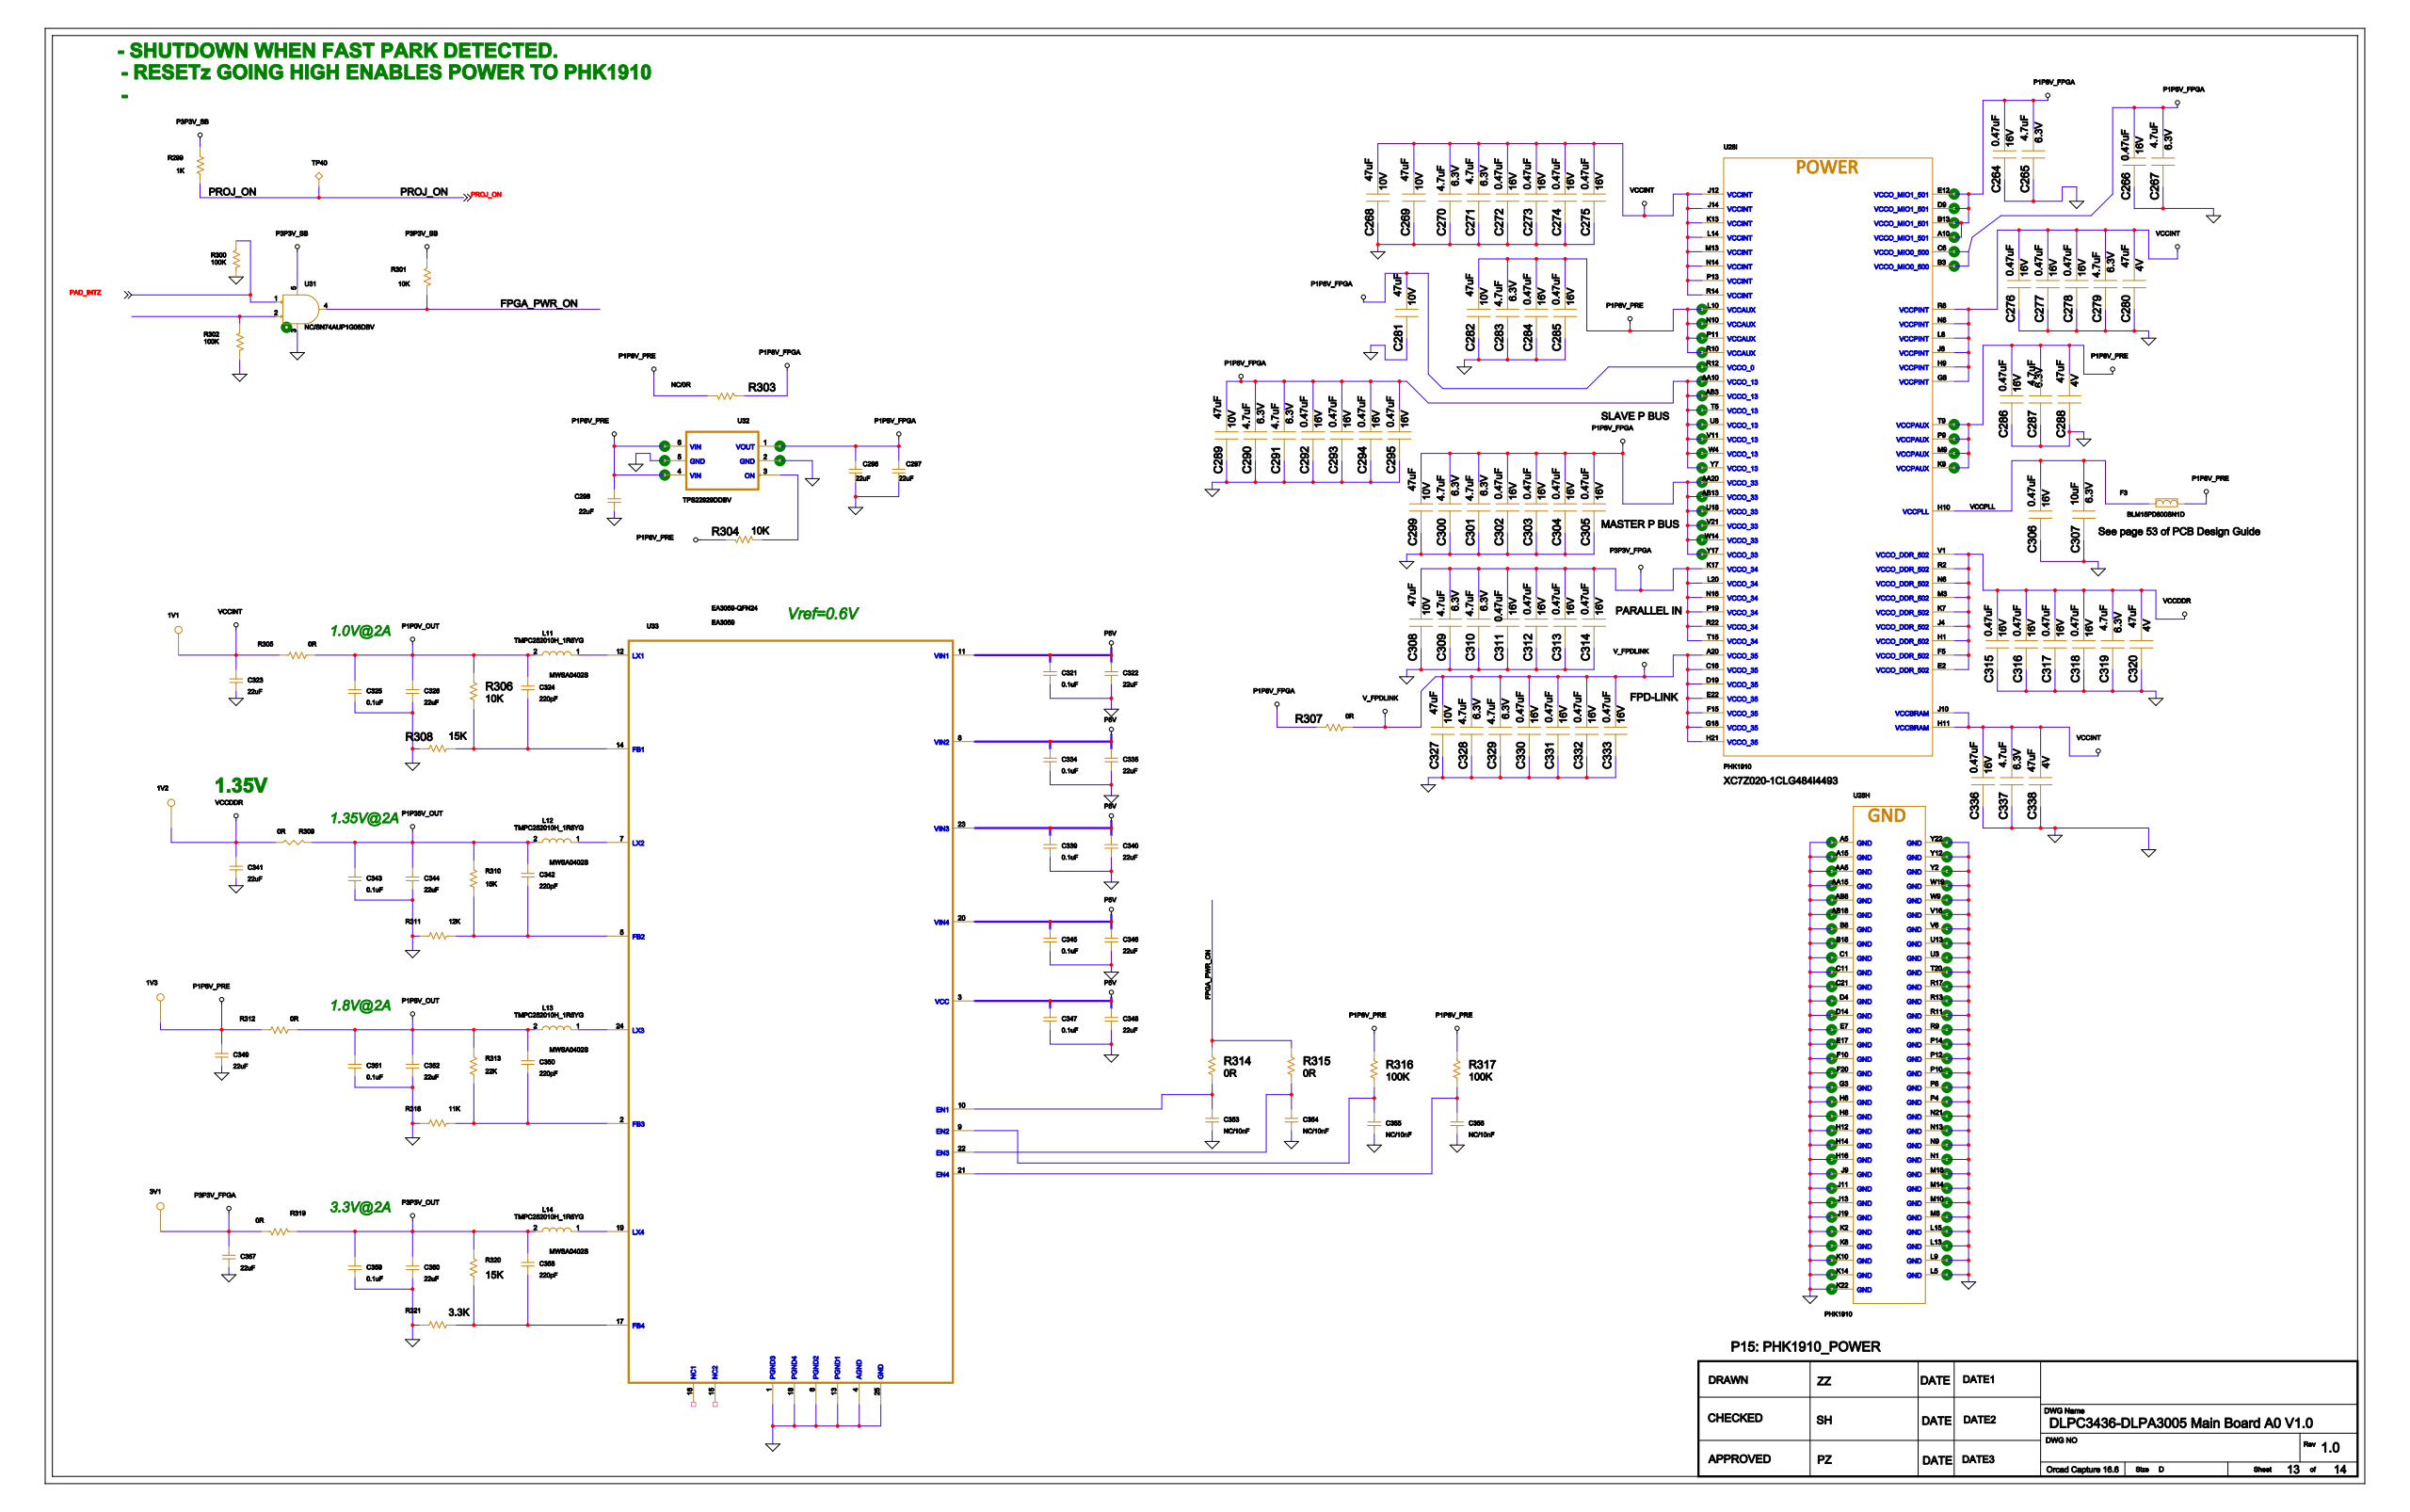Circuit board | Cadence Allegro | 1223 parts | 777 nets | one sheet of the schematic
Parts on this sheet (reference | value | footprint):
1V1 | TP40 | TP06MM
1V2 | TP40 | TP06MM
1V3 | TP40 | TP06MM
3V1 | TP40 | TP06MM
C264 | 0.47uF | C0201
C265 | 4.7uF | C0402
C266 | 0.47uF | C0201
C267 | 4.7uF | C0402
C268 | 47uF | C0805
C269 | 47uF | C0805
C270 | 4.7uF | C0402
C271 | 4.7uF | C0402
C272 | 0.47uF | C0201
C273 | 0.47uF | C0201
C274 | 0.47uF | C0201
C275 | 0.47uF | C0201
C276 | 0.47uF | C0201
C277 | 0.47uF | C0201
C278 | 0.47uF | C0201
C279 | 4.7uF | C0402
C280 | 47uF | C0805
C281 | 47uF | C0805
C282 | 47uF | C0805
C283 | 4.7uF | C0402
C284 | 0.47uF | C0201
C285 | 0.47uF | C0201
C286 | 0.47uF | C0201
C287 | 4.7uF | C0402
C288 | 47uF | C0805
C289 | 47uF | C0805
C290 | 4.7uF | C0402
C291 | 4.7uF | C0402
C292 | 0.47uF | C0201
C293 | 0.47uF | C0201
C294 | 0.47uF | C0201
C295 | 0.47uF | C0201
C296 | 22uF | C0603
C297 | 22uF | C0603
C298 | 22uF | C0603
C299 | 47uF | C0805
C300 | 4.7uF | C0402
C301 | 4.7uF | C0402
C302 | 0.47uF | C0201
C303 | 0.47uF | C0201
C304 | 0.47uF | C0201
C305 | 0.47uF | C0201
C306 | 0.47uF | C0201
C307 | 10uF | C0603
C308 | 47uF | C0805
C309 | 4.7uF | C0402
C310 | 4.7uF | C0402
C311 | 0.47uF | C0201
C312 | 0.47uF | C0201
C313 | 0.47uF | C0201
C314 | 0.47uF | C0201
C315 | 0.47uF | C0201
C316 | 0.47uF | C0201
C317 | 0.47uF | C0201
C318 | 0.47uF | C0201
C319 | 4.7uF | C0402
C320 | 47uF | C0805
C321 | 0.1uF | C0201
C322 | 22uF | C0603
C323 | 22uF | C0603
C324 | 220pF | C0402
C325 | 0.1uF | C0201
C326 | 22uF | C0603
C327 | 47uF | C0805
C328 | 4.7uF | C0402
C329 | 4.7uF | C0402
C330 | 0.47uF | C0201
C331 | 0.47uF | C0201
C332 | 0.47uF | C0201
C333 | 0.47uF | C0201
C334 | 0.1uF | C0201
C335 | 22uF | C0603
C336 | 0.47uF | C0201
C337 | 4.7uF | C0402
C338 | 47uF | C0805
C339 | 0.1uF | C0201
C340 | 22uF | C0603
C341 | 22uF | C0603
C342 | 220pF | C0402
C343 | 0.1uF | C0201
C344 | 22uF | C0603
C345 | 0.1uF | C0201
C346 | 22uF | C0603
C347 | 0.1uF | C0201
C348 | 22uF | C0603
C349 | 22uF | C0603
C350 | 220pF | C0402
C351 | 0.1uF | C0201
C352 | 22uF | C0603
C353 | NC/10nF | C0201
C354 | NC/10nF | C0201
C355 | NC/10nF | C0201
C356 | NC/10nF | C0201
C357 | 22uF | C0603
C358 | 220pF | C0402
C359 | 0.1uF | C0201
C360 | 22uF | C0603
F3 | BLM15PD800SN1D | R0402
L11 | TMPC252010H_1R5YG | MWSA0402S
L12 | TMPC252010H_1R5YG | MWSA0402S
L13 | TMPC252010H_1R5YG | MWSA0402S
L14 | TMPC252010H_1R5YG | MWSA0402S
R299 | 1K | R0201
R300 | 100K | R0201
R301 | 10K | R0201
R302 | 100K | R0201
R303 | NC/0R | R0603
R304 | 10K | R0201
R305 | 0R | R0603
R306 | 10K | R0201
R307 | 0R | R0603
R308 | 15K | R0402
R309 | 0R | R0603
R310 | 15K | R0402
R311 | 12K | R0402
R312 | 0R | R0603
R313 | 22K | R0402
R314 | 0R | R0201
R315 | 0R | R0201
R316 | 100K | R0201
R317 | 100K | R0201
R318 | 11K | R0402
R319 | 0R | R0603
R320 | 15K | R0402
R321 | 3.3K | R0402
TP40 | TP40 | TP06MM
U8 | MT9255 BGA16.4 | LFBGA462
U28 | PHK1910 | XILINX_CLG484
U31 | NC/SN74AUP1G08DBV | SOT25
U32 | TPS22929DDBV | SOT-23-6
U33 | EA3059 | WQFN24_4X4MM
Nets of these parts (net: part-pin ...):
GND: C264-2 C265-2 C266-2 C267-2 C268-2 C269-2 C270-2 C271-2 C272-2 C273-2 C274-2 C275-2 C276-2 C277-2 C278-2 C279-2 C280-2 C281-2 C282-2 C283-2 C284-2 C285-2 C286-2 C287-2 C288-2 C289-2 C290-2 C291-2 C292-2 C293-2 C294-2 C295-2 C296-2 C297-2 C298-1 C299-2 C300-2 C301-2 C302-2 C303-2 C304-2 C305-2 C306-2 C307-2 C308-2 C309-2 C310-2 C311-2 C312-2 C313-2 C314-2 C315-2 C316-2 C317-2 C318-2 C319-2 C320-2 C321-1 C322-1 C323-1 C325-1 C326-1 C327-2 C328-2 C329-2 C330-2 C331-2 C332-2 C333-2 C334-1 C335-1 C336-2 C337-2 C338-2 C339-1 C340-1 C341-1 C343-1 C344-1 C345-1 C346-1 C347-1 C348-1 C349-1 C351-1 C352-1 C353-1 C354-1 C355-1 C356-1 C357-1 C359-1 C360-1 R300-1 R302-1 R308-1 R311-1 R318-1 R321-1 U31-3 U32-2 U32-5 U8-A5 U8-AA10 U8-AA20 U8-AB8 U8-B8 U8-B13 U8-C6 U8-C11 U8-C16 U8-C21 U8-D9 U8-E7 U8-F10 U8-F20 U8-G8 U8-H6 U8-H8 U8-H10 U8-H12 U8-H16 U8-H21 U8-J8 U8-J10 U8-K7 U8-K8 U8-K9 U8-K10 U8-K14 U8-L5 U8-L8 U8-L9 U8-L10 U8-L13 U8-M8 U8-M9 U8-M10 U8-M13 U8-M14 U8-N1 U8-N6 U8-N8 U8-N9 U8-P8 U8-R9 U8-T9 U8-T20 U8-U18 U8-V1 U8-V11 U8-V16 U8-W4 U8-W14 U8-W19 U8-Y7 U8-Y22 U28-A5 U28-A15 U28-AA5 U28-AA15 U28-AB8 U28-AB18 U28-B8 U28-B18 U28-C1 U28-C11 U28-C21 U28-D4 U28-D14 U28-E7 U28-E17 U28-F10 U28-F20 U28-G3 U28-H6 U28-H8 U28-H12 U28-H14 U28-H16 U28-J9 U28-J11 U28-J13 U28-J19 U28-K2 U28-K8 U28-K10 U28-K14 U28-K22 U28-L5 U28-L9 U28-L11 U28-L12 U28-L13 U28-L15 U28-M8 U28-M10 U28-M14 U28-M18 U28-N1 U28-N9 U28-N13 U28-N21 U28-P4 U28-P8 U28-P10 U28-P12 U28-P14 U28-R9 U28-R11 U28-R13 U28-R17 U28-T20 U28-U3 U28-U13 U28-V6 U28-V16 U28-W9 U28-W19 U28-Y2 U28-Y12 U28-Y22 U33-1 U33-4 U33-6 U33-13 U33-18 U33-25
VCCINT: 1V1-1 C268-1 C269-1 C270-1 C271-1 C272-1 C273-1 C274-1 C275-1 C276-1 C277-1 C278-1 C279-1 C280-1 C323-2 C336-1 C337-1 C338-1 R305-2 U28-G8 U28-H9 U28-H11 U28-J8 U28-J10 U28-J12 U28-J14 U28-K13 U28-L8 U28-L14 U28-M13 U28-N8 U28-N14 U28-P13 U28-R8 U28-R14
VCCDDR: 1V2-1 C315-1 C316-1 C317-1 C318-1 C319-1 C320-1 C341-2 R309-2 U28-E2 U28-F5 U28-H1 U28-J4 U28-K7 U28-M3 U28-N6 U28-R2 U28-V1
P1P8V_PRE: 1V3-1 C282-1 C283-1 C284-1 C285-1 C286-1 C287-1 C288-1 C298-2 C349-2 F3-2 R303-1 R304-2 R312-2 R316-2 R317-2 U32-4 U32-6 U28-K9 U28-L10 U28-M9 U28-N10 U28-P9 U28-P11 U28-R10 U28-T9
P3P3V_FPGA: 3V1-1 C308-1 C309-1 C310-1 C311-1 C312-1 C313-1 C314-1 C357-2 R319-1 U28-K17 U28-L20 U28-N16 U28-P19 U28-R22 U28-T15
P3P3V_SB: R299-1 R301-2 U31-5
P1P8V_FPGA: C264-1 C265-1 C266-1 C267-1 C281-1 C289-1 C290-1 C291-1 C292-1 C293-1 C294-1 C295-1 C296-1 C297-1 C299-1 C300-1 C301-1 C302-1 C303-1 C304-1 C305-1 R303-2 R307-2 U32-1 U28-A10 U28-AA10 U28-AA20 U28-AB3 U28-AB13 U28-B3 U28-B13 U28-C6 U28-D9 U28-E12 U28-R12 U28-T5 U28-U8 U28-U18 U28-V11 U28-V21 U28-W4 U28-W14 U28-Y7 U28-Y17
P5V: C321-2 C322-2 C334-2 C335-2 C339-2 C340-2 C345-2 C346-2 C347-2 C348-2 U33-3 U33-8 U33-11 U33-20 U33-23
VCCPLL: C306-1 C307-1 F3-1 U28-H10
V_FPDLINK: C327-1 C328-1 C329-1 C330-1 C331-1 C332-1 C333-1 R307-1 U28-A20 U28-C16 U28-D19 U28-E22 U28-F15 U28-G18 U28-H21
P1P0V_OUT: C324-2 C325-2 C326-2 L11-2 R305-1 R306-2
P1P35V_OUT: C342-2 C343-2 C344-2 L12-2 R309-1 R310-2
P1P8V_OUT: C350-2 C351-2 C352-2 L13-2 R312-1 R313-2
P3P3V_OUT: C358-2 C359-2 C360-2 L14-2 R319-2 R320-2
N23924312: C324-1 R306-1 R308-2 U33-14
N23923428: C342-1 R310-1 R311-2 U33-5
N23923547: C350-1 R313-1 R318-2 U33-2
N23923641: C358-1 R320-1 R321-2 U33-17
N23923977: C353-2 R314-1 U33-10
N23924005: C354-2 R315-1 U33-22
N23924069: C355-2 R316-1 U33-9
N23924035: C356-2 R317-1 U33-21
PAD_INTZ: R300-2 U31-1
PROJ_ON: R299-2 TP40-1
N23924293: L11-1 U33-12
N23923430: L12-1 U33-7
N23923522: L13-1 U33-24
N23923617: L14-1 U33-19
N22225935: R302-2 U31-2
FPGA_PWR_ON: R301-1 R314-2 R315-2 U31-4
N23925787: R304-1 U32-3